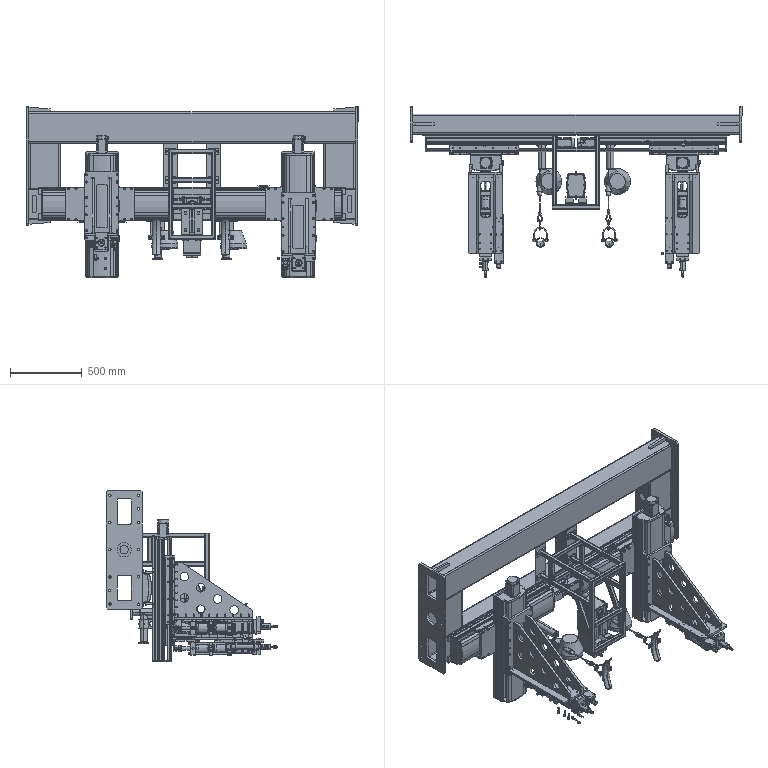Part | SolidWorks | 509 solids | 16947 faces | volume 116635153 mm3 | plane 7361 | cylinder 6709 | cone 1673 | torus 812 | spline 336 | sphere 56 | commonest cylinder face diameters 15 x584 6.8 x520 8 x356 9 x342 8.6 x336 13 x278